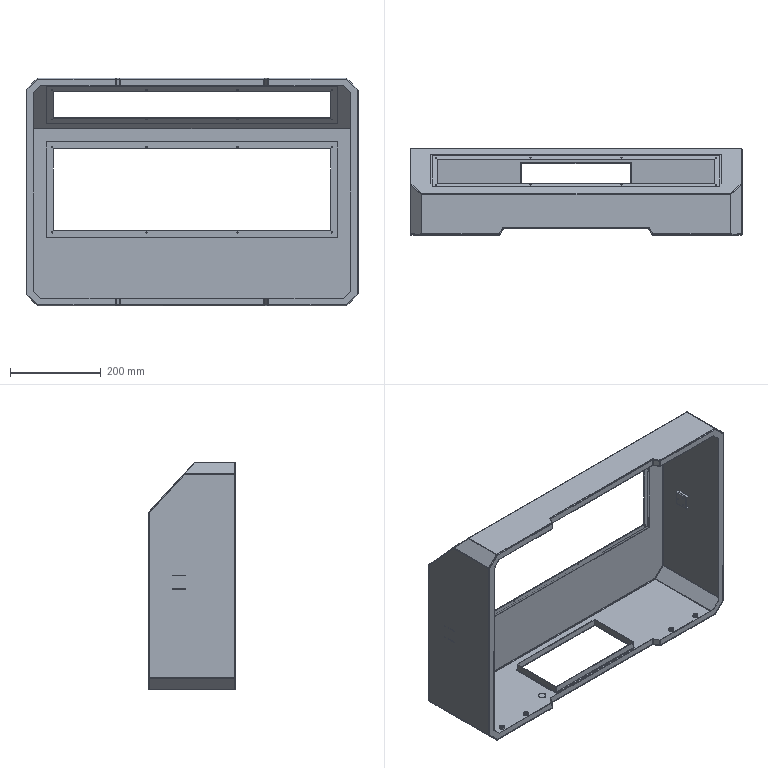Part | SolidWorks | features BaseBody 1 | 1 solid | 347 faces | box 730 x 190 x 500 mm | volume 771192 mm3 | cylinder 178 | plane 109 | sphere 36 | spline 16 | torus 8 | commonest cylinder face diameters 4 x51 2.5 x44 2 x40 1.6 x19 5 x8 11 x8